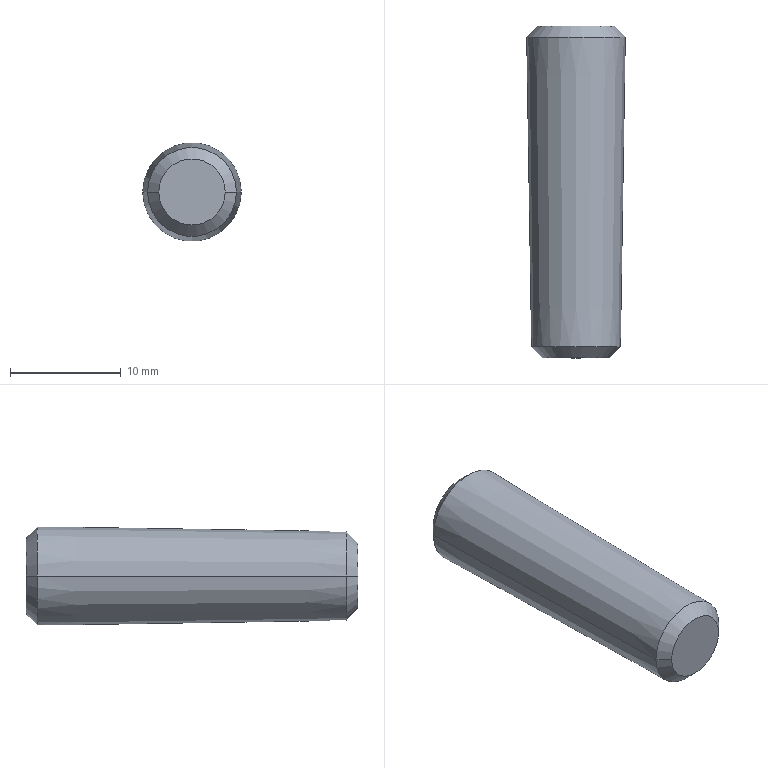Part | NX | features BREP 1 | 1 solid | 8 faces | box 8.911 x 30 x 8.911 mm | volume 1668 mm3 | cone 6 | plane 2
STEP:
#1=CARTESIAN_POINT('',(3.,-30.,0.));
#2=VERTEX_POINT('',#1);
#3=CARTESIAN_POINT('',(-3.,-30.,0.));
#4=VERTEX_POINT('',#3);
#5=CARTESIAN_POINT('',(0.,-30.,0.));
#6=DIRECTION('',(0.,1.,0.));
#7=DIRECTION('',(1.,0.,0.));
#8=AXIS2_PLACEMENT_3D('',#5,#6,#7);
#9=CIRCLE('',#8,3.);
#10=EDGE_CURVE('',#2,#4,#9,.T.);
#11=ORIENTED_EDGE('',*,*,#10,.F.);
#12=CARTESIAN_POINT('',(0.,-30.,0.));
#13=DIRECTION('',(0.,-1.,0.));
#14=DIRECTION('',(1.,0.,0.));
#15=AXIS2_PLACEMENT_3D('',#12,#13,#14);
#16=CIRCLE('',#15,3.);
#17=EDGE_CURVE('',#2,#4,#16,.T.);
#18=ORIENTED_EDGE('',*,*,#17,.T.);
#19=EDGE_LOOP('',(#11,#18));
#20=FACE_BOUND('',#19,.T.);
#21=CARTESIAN_POINT('',(0.,-30.,0.));
#22=DIRECTION('',(0.,1.,0.));
#23=DIRECTION('',(-1.,0.,0.));
#24=AXIS2_PLACEMENT_3D('',#21,#22,#23);
#25=PLANE('',#24);
#26=ADVANCED_FACE('',(#20),#25,.F.);
#27=CARTESIAN_POINT('',(-4.016,-29.,0.));
#28=VERTEX_POINT('',#27);
#29=CARTESIAN_POINT('',(-4.016,-29.,0.));
#30=DIRECTION('',(0.7126,-0.7015,0.));
#31=VECTOR('',#30,1000.);
#32=LINE('',#29,#31);
#33=EDGE_CURVE('',#28,#4,#32,.T.);
#34=ORIENTED_EDGE('',*,*,#33,.T.);
#35=ORIENTED_EDGE('',*,*,#17,.F.);
#36=CARTESIAN_POINT('',(4.016,-29.,0.));
#37=VERTEX_POINT('',#36);
#38=CARTESIAN_POINT('',(4.016,-29.,0.));
#39=DIRECTION('',(-0.7126,-0.7015,0.));
#40=VECTOR('',#39,1000.);
#41=LINE('',#38,#40);
#42=EDGE_CURVE('',#37,#2,#41,.T.);
#43=ORIENTED_EDGE('',*,*,#42,.F.);
#44=CARTESIAN_POINT('',(0.,-29.,0.));
#45=DIRECTION('',(0.,-1.,0.));
#46=DIRECTION('',(1.,0.,0.));
#47=AXIS2_PLACEMENT_3D('',#44,#45,#46);
#48=CIRCLE('',#47,4.016);
#49=EDGE_CURVE('',#37,#28,#48,.T.);
#50=ORIENTED_EDGE('',*,*,#49,.T.);
#51=EDGE_LOOP('',(#34,#35,#43,#50));
#52=FACE_BOUND('',#51,.T.);
#53=CARTESIAN_POINT('',(0.,-29.5,0.));
#54=DIRECTION('',(0.,1.,0.));
#55=DIRECTION('',(-1.,0.,0.));
#56=AXIS2_PLACEMENT_3D('',#53,#54,#55);
#57=CONICAL_SURFACE('',#56,3.508,0.7933);
#58=ADVANCED_FACE('',(#52),#57,.T.);
#59=CARTESIAN_POINT('',(4.456,-0.9999,0.));
#60=VERTEX_POINT('',#59);
#61=CARTESIAN_POINT('',(-4.456,-0.9999,0.));
#62=VERTEX_POINT('',#61);
#63=CARTESIAN_POINT('',(0.,-0.9999,0.));
#64=DIRECTION('',(0.,-1.,0.));
#65=DIRECTION('',(1.,0.,0.));
#66=AXIS2_PLACEMENT_3D('',#63,#64,#65);
#67=CIRCLE('',#66,4.456);
#68=EDGE_CURVE('',#60,#62,#67,.T.);
#69=ORIENTED_EDGE('',*,*,#68,.T.);
#70=CARTESIAN_POINT('',(-4.016,-29.,0.));
#71=DIRECTION('',(-0.01571,0.9999,0.));
#72=VECTOR('',#71,1000.);
#73=LINE('',#70,#72);
#74=EDGE_CURVE('',#62,#28,#73,.F.);
#75=ORIENTED_EDGE('',*,*,#74,.T.);
#76=ORIENTED_EDGE('',*,*,#49,.F.);
#77=CARTESIAN_POINT('',(4.016,-29.,0.));
#78=DIRECTION('',(0.01571,0.9999,0.));
#79=VECTOR('',#78,1000.);
#80=LINE('',#77,#79);
#81=EDGE_CURVE('',#60,#37,#80,.F.);
#82=ORIENTED_EDGE('',*,*,#81,.F.);
#83=EDGE_LOOP('',(#69,#75,#76,#82));
#84=FACE_BOUND('',#83,.T.);
#85=CARTESIAN_POINT('',(0.,-15.,0.));
#86=DIRECTION('',(0.,1.,0.));
#87=DIRECTION('',(-1.,0.,0.));
#88=AXIS2_PLACEMENT_3D('',#85,#86,#87);
#89=CONICAL_SURFACE('',#88,4.236,0.01571);
#90=ADVANCED_FACE('',(#84),#89,.T.);
#91=CARTESIAN_POINT('',(0.,-29.,0.));
#92=DIRECTION('',(0.,1.,0.));
#93=DIRECTION('',(1.,0.,0.));
#94=AXIS2_PLACEMENT_3D('',#91,#92,#93);
#95=CIRCLE('',#94,4.016);
#96=EDGE_CURVE('',#37,#28,#95,.T.);
#97=ORIENTED_EDGE('',*,*,#96,.T.);
#98=ORIENTED_EDGE('',*,*,#74,.F.);
#99=CARTESIAN_POINT('',(0.,-0.9999,0.));
#100=DIRECTION('',(0.,1.,0.));
#101=DIRECTION('',(1.,0.,0.));
#102=AXIS2_PLACEMENT_3D('',#99,#100,#101);
#103=CIRCLE('',#102,4.456);
#104=EDGE_CURVE('',#60,#62,#103,.T.);
#105=ORIENTED_EDGE('',*,*,#104,.F.);
#106=ORIENTED_EDGE('',*,*,#81,.T.);
#107=EDGE_LOOP('',(#97,#98,#105,#106));
#108=FACE_BOUND('',#107,.T.);
#109=CARTESIAN_POINT('',(0.,-15.,0.));
#110=DIRECTION('',(0.,1.,0.));
#111=DIRECTION('',(-1.,0.,0.));
#112=AXIS2_PLACEMENT_3D('',#109,#110,#111);
#113=CONICAL_SURFACE('',#112,4.236,0.01571);
#114=ADVANCED_FACE('',(#108),#113,.T.);
#115=CARTESIAN_POINT('',(3.471,0.,0.));
#116=VERTEX_POINT('',#115);
#117=CARTESIAN_POINT('',(3.471,0.,0.));
#118=DIRECTION('',(0.7015,-0.7126,0.));
#119=VECTOR('',#118,1000.);
#120=LINE('',#117,#119);
#121=EDGE_CURVE('',#60,#116,#120,.F.);
#122=ORIENTED_EDGE('',*,*,#121,.F.);
#123=ORIENTED_EDGE('',*,*,#104,.T.);
#124=CARTESIAN_POINT('',(-3.471,0.,0.));
#125=VERTEX_POINT('',#124);
#126=CARTESIAN_POINT('',(-3.471,0.,0.));
#127=DIRECTION('',(-0.7015,-0.7126,0.));
#128=VECTOR('',#127,1000.);
#129=LINE('',#126,#128);
#130=EDGE_CURVE('',#62,#125,#129,.F.);
#131=ORIENTED_EDGE('',*,*,#130,.T.);
#132=CARTESIAN_POINT('',(0.,0.,0.));
#133=DIRECTION('',(0.,1.,0.));
#134=DIRECTION('',(1.,0.,0.));
#135=AXIS2_PLACEMENT_3D('',#132,#133,#134);
#136=CIRCLE('',#135,3.471);
#137=EDGE_CURVE('',#116,#125,#136,.T.);
#138=ORIENTED_EDGE('',*,*,#137,.F.);
#139=EDGE_LOOP('',(#122,#123,#131,#138));
#140=FACE_BOUND('',#139,.T.);
#141=CARTESIAN_POINT('',(0.,-0.4999,0.));
#142=DIRECTION('',(0.,-1.,0.));
#143=DIRECTION('',(1.,0.,0.));
#144=AXIS2_PLACEMENT_3D('',#141,#142,#143);
#145=CONICAL_SURFACE('',#144,3.963,0.7775);
#146=ADVANCED_FACE('',(#140),#145,.T.);
#147=ORIENTED_EDGE('',*,*,#137,.T.);
#148=CARTESIAN_POINT('',(0.,0.,0.));
#149=DIRECTION('',(0.,-1.,0.));
#150=DIRECTION('',(1.,0.,0.));
#151=AXIS2_PLACEMENT_3D('',#148,#149,#150);
#152=CIRCLE('',#151,3.471);
#153=EDGE_CURVE('',#116,#125,#152,.T.);
#154=ORIENTED_EDGE('',*,*,#153,.F.);
#155=EDGE_LOOP('',(#147,#154));
#156=FACE_BOUND('',#155,.T.);
#157=CARTESIAN_POINT('',(0.,0.,0.));
#158=DIRECTION('',(0.,1.,0.));
#159=DIRECTION('',(-1.,0.,0.));
#160=AXIS2_PLACEMENT_3D('',#157,#158,#159);
#161=PLANE('',#160);
#162=ADVANCED_FACE('',(#156),#161,.T.);
#163=ORIENTED_EDGE('',*,*,#130,.F.);
#164=ORIENTED_EDGE('',*,*,#68,.F.);
#165=ORIENTED_EDGE('',*,*,#121,.T.);
#166=ORIENTED_EDGE('',*,*,#153,.T.);
#167=EDGE_LOOP('',(#163,#164,#165,#166));
#168=FACE_BOUND('',#167,.T.);
#169=CARTESIAN_POINT('',(0.,-0.4999,0.));
#170=DIRECTION('',(0.,-1.,0.));
#171=DIRECTION('',(1.,0.,0.));
#172=AXIS2_PLACEMENT_3D('',#169,#170,#171);
#173=CONICAL_SURFACE('',#172,3.963,0.7775);
#174=ADVANCED_FACE('',(#168),#173,.T.);
#175=ORIENTED_EDGE('',*,*,#42,.T.);
#176=ORIENTED_EDGE('',*,*,#10,.T.);
#177=ORIENTED_EDGE('',*,*,#33,.F.);
#178=ORIENTED_EDGE('',*,*,#96,.F.);
#179=EDGE_LOOP('',(#175,#176,#177,#178));
#180=FACE_BOUND('',#179,.T.);
#181=CARTESIAN_POINT('',(0.,-29.5,0.));
#182=DIRECTION('',(0.,1.,0.));
#183=DIRECTION('',(-1.,0.,0.));
#184=AXIS2_PLACEMENT_3D('',#181,#182,#183);
#185=CONICAL_SURFACE('',#184,3.508,0.7933);
#186=ADVANCED_FACE('',(#180),#185,.T.);
#187=CLOSED_SHELL('',(#26,#58,#90,#114,#146,#162,#174,#186));
#188=MANIFOLD_SOLID_BREP('',#187);
#189=(LENGTH_UNIT()NAMED_UNIT(*)SI_UNIT(.MILLI.,.METRE.));
#190=UNCERTAINTY_MEASURE_WITH_UNIT(LENGTH_MEASURE(0.00001),#189,'','');
#191=(NAMED_UNIT(*)PLANE_ANGLE_UNIT()SI_UNIT($,.RADIAN.));
#192=(NAMED_UNIT(*)SI_UNIT($,.STERADIAN.)SOLID_ANGLE_UNIT());
#193=(GEOMETRIC_REPRESENTATION_CONTEXT(3)GLOBAL_UNCERTAINTY_ASSIGNED_CONTEXT((#190))GLOBAL_UNIT_ASSIGNED_CONTEXT((#189,#191,#192))REPRESENTATION_CONTEXT('',''));
#194=ADVANCED_BREP_SHAPE_REPRESENTATION('',(#188),#193);